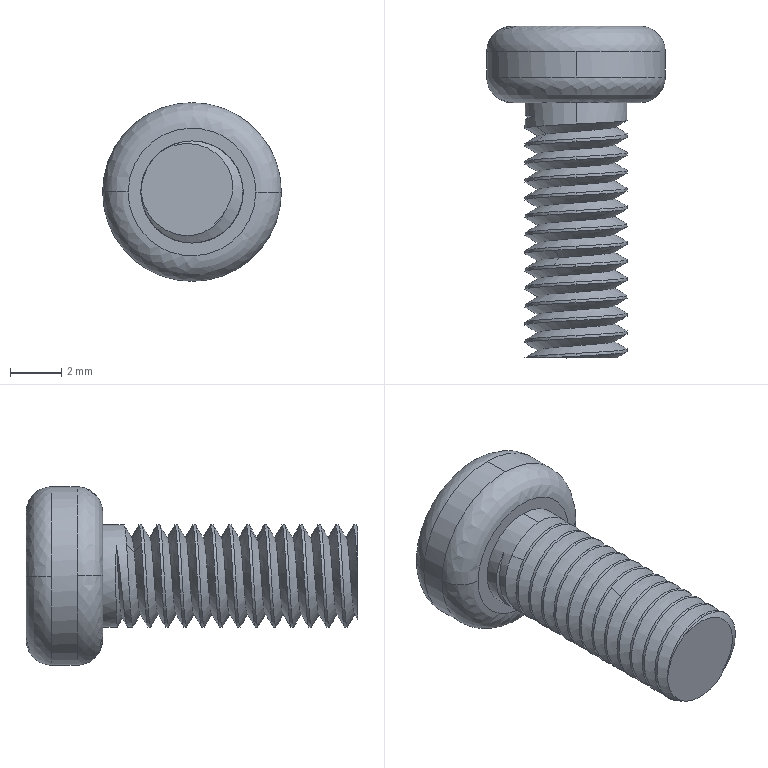Part | STEP file | 1 solid | 64 faces | box 7 x 13 x 7 mm | volume 186.803 mm3 | cylinder 34 | plane 16 | spline 14 | commonest cylinder face diameters 4 x28 0.8 x4 7 x2